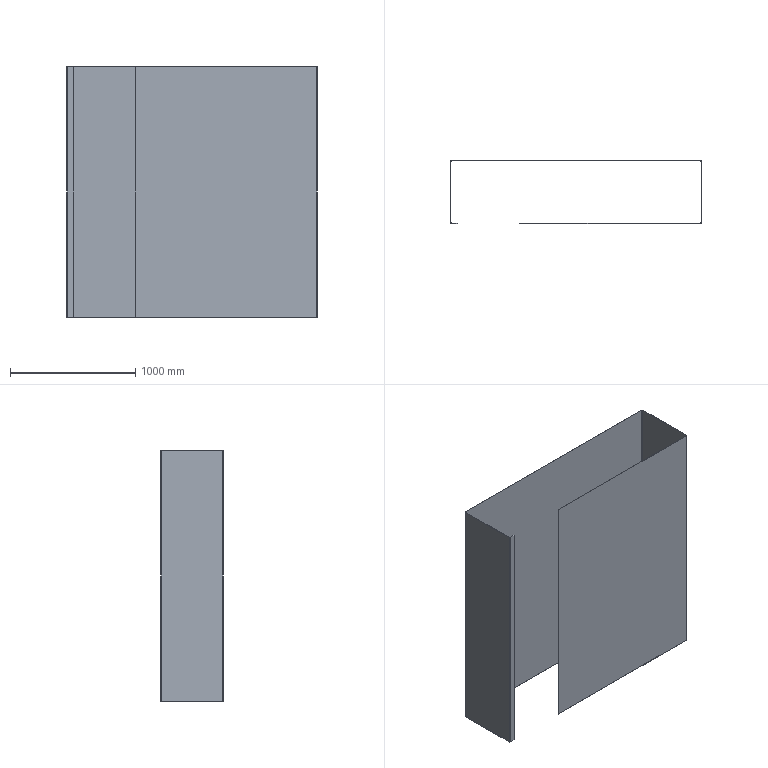Part | SolidWorks | features BaseBody 1 | 1 solid | 38 faces | box 2003 x 503 x 2000 mm | volume 13488385 mm3 | plane 30 | cylinder 8 | commonest cylinder face diameters 10 x4 13 x4
STEP:
#1=CARTESIAN_POINT('',(-995.,-500.,2000.));
#2=VERTEX_POINT('',#1);
#3=CARTESIAN_POINT('',(-995.,-501.5,2000.));
#4=VERTEX_POINT('',#3);
#5=CARTESIAN_POINT('',(-995.,-500.,2000.));
#6=DIRECTION('',(0.,-1.,0.));
#7=VECTOR('',#6,1000.);
#8=LINE('',#5,#7);
#9=EDGE_CURVE('',#2,#4,#8,.T.);
#10=ORIENTED_EDGE('',*,*,#9,.F.);
#11=CARTESIAN_POINT('',(-1000.,-495.,2000.));
#12=VERTEX_POINT('',#11);
#13=CARTESIAN_POINT('',(-995.,-495.,2000.));
#14=DIRECTION('',(0.,0.,1.));
#15=DIRECTION('',(1.,0.,0.));
#16=AXIS2_PLACEMENT_3D('',#13,#14,#15);
#17=CIRCLE('',#16,5.);
#18=EDGE_CURVE('',#12,#2,#17,.T.);
#19=ORIENTED_EDGE('',*,*,#18,.F.);
#20=CARTESIAN_POINT('',(-1001.5,-495.,2000.));
#21=VERTEX_POINT('',#20);
#22=CARTESIAN_POINT('',(-1001.5,-495.,2000.));
#23=DIRECTION('',(1.,0.,0.));
#24=VECTOR('',#23,1000.);
#25=LINE('',#22,#24);
#26=EDGE_CURVE('',#21,#12,#25,.T.);
#27=ORIENTED_EDGE('',*,*,#26,.F.);
#28=CARTESIAN_POINT('',(-995.,-495.,2000.));
#29=DIRECTION('',(0.,0.,1.));
#30=DIRECTION('',(1.,0.,0.));
#31=AXIS2_PLACEMENT_3D('',#28,#29,#30);
#32=CIRCLE('',#31,6.5);
#33=EDGE_CURVE('',#21,#4,#32,.T.);
#34=ORIENTED_EDGE('',*,*,#33,.T.);
#35=EDGE_LOOP('',(#10,#19,#27,#34));
#36=FACE_OUTER_BOUND('',#35,.T.);
#37=CARTESIAN_POINT('',(-995.,-500.,2000.));
#38=DIRECTION('',(0.,0.,1.));
#39=DIRECTION('',(1.,0.,0.));
#40=AXIS2_PLACEMENT_3D('',#37,#38,#39);
#41=PLANE('',#40);
#42=ADVANCED_FACE('',(#36),#41,.T.);
#43=CARTESIAN_POINT('',(-950.,-500.,2000.));
#44=VERTEX_POINT('',#43);
#45=CARTESIAN_POINT('',(-995.,-500.,2000.));
#46=DIRECTION('',(1.,0.,0.));
#47=VECTOR('',#46,1000.);
#48=LINE('',#45,#47);
#49=EDGE_CURVE('',#2,#44,#48,.T.);
#50=ORIENTED_EDGE('',*,*,#49,.F.);
#51=ORIENTED_EDGE('',*,*,#9,.T.);
#52=CARTESIAN_POINT('',(-950.,-501.5,2000.));
#53=VERTEX_POINT('',#52);
#54=CARTESIAN_POINT('',(-995.,-501.5,2000.));
#55=DIRECTION('',(1.,0.,0.));
#56=VECTOR('',#55,1000.);
#57=LINE('',#54,#56);
#58=EDGE_CURVE('',#4,#53,#57,.T.);
#59=ORIENTED_EDGE('',*,*,#58,.T.);
#60=CARTESIAN_POINT('',(-950.,-500.,2000.));
#61=DIRECTION('',(0.,-1.,0.));
#62=VECTOR('',#61,1000.);
#63=LINE('',#60,#62);
#64=EDGE_CURVE('',#44,#53,#63,.T.);
#65=ORIENTED_EDGE('',*,*,#64,.F.);
#66=EDGE_LOOP('',(#50,#51,#59,#65));
#67=FACE_OUTER_BOUND('',#66,.T.);
#68=CARTESIAN_POINT('',(-1001.5,-495.,2000.));
#69=DIRECTION('',(0.,0.,1.));
#70=DIRECTION('',(1.,0.,0.));
#71=AXIS2_PLACEMENT_3D('',#68,#69,#70);
#72=PLANE('',#71);
#73=ADVANCED_FACE('',(#67),#72,.T.);
#74=CARTESIAN_POINT('',(-1000.,-495.,0.));
#75=VERTEX_POINT('',#74);
#76=CARTESIAN_POINT('',(-1001.5,-495.,0.));
#77=VERTEX_POINT('',#76);
#78=CARTESIAN_POINT('',(-1000.,-495.,0.));
#79=DIRECTION('',(-1.,0.,0.));
#80=VECTOR('',#79,1000.);
#81=LINE('',#78,#80);
#82=EDGE_CURVE('',#75,#77,#81,.T.);
#83=ORIENTED_EDGE('',*,*,#82,.F.);
#84=CARTESIAN_POINT('',(-995.,-500.,0.));
#85=VERTEX_POINT('',#84);
#86=CARTESIAN_POINT('',(-995.,-495.,0.));
#87=DIRECTION('',(0.,0.,1.));
#88=DIRECTION('',(1.,0.,0.));
#89=AXIS2_PLACEMENT_3D('',#86,#87,#88);
#90=CIRCLE('',#89,5.);
#91=EDGE_CURVE('',#75,#85,#90,.T.);
#92=ORIENTED_EDGE('',*,*,#91,.T.);
#93=CARTESIAN_POINT('',(-995.,-501.5,0.));
#94=VERTEX_POINT('',#93);
#95=CARTESIAN_POINT('',(-995.,-501.5,0.));
#96=DIRECTION('',(0.,1.,0.));
#97=VECTOR('',#96,1000.);
#98=LINE('',#95,#97);
#99=EDGE_CURVE('',#94,#85,#98,.T.);
#100=ORIENTED_EDGE('',*,*,#99,.F.);
#101=CARTESIAN_POINT('',(-995.,-495.,0.));
#102=DIRECTION('',(0.,0.,1.));
#103=DIRECTION('',(1.,0.,0.));
#104=AXIS2_PLACEMENT_3D('',#101,#102,#103);
#105=CIRCLE('',#104,6.5);
#106=EDGE_CURVE('',#77,#94,#105,.T.);
#107=ORIENTED_EDGE('',*,*,#106,.F.);
#108=EDGE_LOOP('',(#83,#92,#100,#107));
#109=FACE_OUTER_BOUND('',#108,.T.);
#110=CARTESIAN_POINT('',(-1000.,-495.,0.));
#111=DIRECTION('',(0.,0.,-1.));
#112=DIRECTION('',(-1.,0.,0.));
#113=AXIS2_PLACEMENT_3D('',#110,#111,#112);
#114=PLANE('',#113);
#115=ADVANCED_FACE('',(#109),#114,.T.);
#116=CARTESIAN_POINT('',(-1000.,-5.,0.));
#117=VERTEX_POINT('',#116);
#118=CARTESIAN_POINT('',(-1000.,-5.,0.));
#119=DIRECTION('',(0.,-1.,0.));
#120=VECTOR('',#119,1000.);
#121=LINE('',#118,#120);
#122=EDGE_CURVE('',#117,#75,#121,.T.);
#123=ORIENTED_EDGE('',*,*,#122,.T.);
#124=ORIENTED_EDGE('',*,*,#82,.T.);
#125=CARTESIAN_POINT('',(-1001.5,-5.,0.));
#126=VERTEX_POINT('',#125);
#127=CARTESIAN_POINT('',(-1001.5,-5.,0.));
#128=DIRECTION('',(0.,-1.,0.));
#129=VECTOR('',#128,1000.);
#130=LINE('',#127,#129);
#131=EDGE_CURVE('',#126,#77,#130,.T.);
#132=ORIENTED_EDGE('',*,*,#131,.F.);
#133=CARTESIAN_POINT('',(-1001.5,-5.,0.));
#134=DIRECTION('',(1.,0.,0.));
#135=VECTOR('',#134,1000.);
#136=LINE('',#133,#135);
#137=EDGE_CURVE('',#126,#117,#136,.T.);
#138=ORIENTED_EDGE('',*,*,#137,.T.);
#139=EDGE_LOOP('',(#123,#124,#132,#138));
#140=FACE_OUTER_BOUND('',#139,.T.);
#141=CARTESIAN_POINT('',(-995.,-501.5,0.));
#142=DIRECTION('',(0.,0.,-1.));
#143=DIRECTION('',(-1.,0.,0.));
#144=AXIS2_PLACEMENT_3D('',#141,#142,#143);
#145=PLANE('',#144);
#146=ADVANCED_FACE('',(#140),#145,.T.);
#147=CARTESIAN_POINT('',(-1000.,-5.,2000.));
#148=VERTEX_POINT('',#147);
#149=CARTESIAN_POINT('',(-1001.5,-5.,2000.));
#150=VERTEX_POINT('',#149);
#151=CARTESIAN_POINT('',(-1000.,-5.,2000.));
#152=DIRECTION('',(-1.,0.,0.));
#153=VECTOR('',#152,1000.);
#154=LINE('',#151,#153);
#155=EDGE_CURVE('',#148,#150,#154,.T.);
#156=ORIENTED_EDGE('',*,*,#155,.F.);
#157=CARTESIAN_POINT('',(-995.,0.,2000.));
#158=VERTEX_POINT('',#157);
#159=CARTESIAN_POINT('',(-995.,-5.,2000.));
#160=DIRECTION('',(0.,0.,1.));
#161=DIRECTION('',(1.,0.,0.));
#162=AXIS2_PLACEMENT_3D('',#159,#160,#161);
#163=CIRCLE('',#162,5.);
#164=EDGE_CURVE('',#158,#148,#163,.T.);
#165=ORIENTED_EDGE('',*,*,#164,.F.);
#166=CARTESIAN_POINT('',(-995.,1.5,2000.));
#167=VERTEX_POINT('',#166);
#168=CARTESIAN_POINT('',(-995.,1.5,2000.));
#169=DIRECTION('',(0.,-1.,0.));
#170=VECTOR('',#169,1000.);
#171=LINE('',#168,#170);
#172=EDGE_CURVE('',#167,#158,#171,.T.);
#173=ORIENTED_EDGE('',*,*,#172,.F.);
#174=CARTESIAN_POINT('',(-995.,-5.,2000.));
#175=DIRECTION('',(0.,0.,1.));
#176=DIRECTION('',(1.,0.,0.));
#177=AXIS2_PLACEMENT_3D('',#174,#175,#176);
#178=CIRCLE('',#177,6.5);
#179=EDGE_CURVE('',#167,#150,#178,.T.);
#180=ORIENTED_EDGE('',*,*,#179,.T.);
#181=EDGE_LOOP('',(#156,#165,#173,#180));
#182=FACE_OUTER_BOUND('',#181,.T.);
#183=CARTESIAN_POINT('',(-1000.,-5.,2000.));
#184=DIRECTION('',(0.,0.,1.));
#185=DIRECTION('',(1.,0.,0.));
#186=AXIS2_PLACEMENT_3D('',#183,#184,#185);
#187=PLANE('',#186);
#188=ADVANCED_FACE('',(#182),#187,.T.);
#189=CARTESIAN_POINT('',(-1000.,-5.,2000.));
#190=DIRECTION('',(0.,-1.,0.));
#191=VECTOR('',#190,1000.);
#192=LINE('',#189,#191);
#193=EDGE_CURVE('',#148,#12,#192,.T.);
#194=ORIENTED_EDGE('',*,*,#193,.F.);
#195=ORIENTED_EDGE('',*,*,#155,.T.);
#196=CARTESIAN_POINT('',(-1001.5,-5.,2000.));
#197=DIRECTION('',(0.,-1.,0.));
#198=VECTOR('',#197,1000.);
#199=LINE('',#196,#198);
#200=EDGE_CURVE('',#150,#21,#199,.T.);
#201=ORIENTED_EDGE('',*,*,#200,.T.);
#202=ORIENTED_EDGE('',*,*,#26,.T.);
#203=EDGE_LOOP('',(#194,#195,#201,#202));
#204=FACE_OUTER_BOUND('',#203,.T.);
#205=CARTESIAN_POINT('',(-995.,1.5,2000.));
#206=DIRECTION('',(0.,0.,1.));
#207=DIRECTION('',(1.,0.,0.));
#208=AXIS2_PLACEMENT_3D('',#205,#206,#207);
#209=PLANE('',#208);
#210=ADVANCED_FACE('',(#204),#209,.T.);
#211=CARTESIAN_POINT('',(-995.,0.,0.));
#212=VERTEX_POINT('',#211);
#213=CARTESIAN_POINT('',(-995.,1.5,0.));
#214=VERTEX_POINT('',#213);
#215=CARTESIAN_POINT('',(-995.,0.,0.));
#216=DIRECTION('',(0.,1.,0.));
#217=VECTOR('',#216,1000.);
#218=LINE('',#215,#217);
#219=EDGE_CURVE('',#212,#214,#218,.T.);
#220=ORIENTED_EDGE('',*,*,#219,.F.);
#221=CARTESIAN_POINT('',(-995.,-5.,0.));
#222=DIRECTION('',(0.,0.,1.));
#223=DIRECTION('',(1.,0.,0.));
#224=AXIS2_PLACEMENT_3D('',#221,#222,#223);
#225=CIRCLE('',#224,5.);
#226=EDGE_CURVE('',#212,#117,#225,.T.);
#227=ORIENTED_EDGE('',*,*,#226,.T.);
#228=ORIENTED_EDGE('',*,*,#137,.F.);
#229=CARTESIAN_POINT('',(-995.,-5.,0.));
#230=DIRECTION('',(0.,0.,1.));
#231=DIRECTION('',(1.,0.,0.));
#232=AXIS2_PLACEMENT_3D('',#229,#230,#231);
#233=CIRCLE('',#232,6.5);
#234=EDGE_CURVE('',#214,#126,#233,.T.);
#235=ORIENTED_EDGE('',*,*,#234,.F.);
#236=EDGE_LOOP('',(#220,#227,#228,#235));
#237=FACE_OUTER_BOUND('',#236,.T.);
#238=CARTESIAN_POINT('',(-995.,0.,0.));
#239=DIRECTION('',(0.,0.,-1.));
#240=DIRECTION('',(-1.,0.,0.));
#241=AXIS2_PLACEMENT_3D('',#238,#239,#240);
#242=PLANE('',#241);
#243=ADVANCED_FACE('',(#237),#242,.T.);
#244=CARTESIAN_POINT('',(995.,0.,0.));
#245=VERTEX_POINT('',#244);
#246=CARTESIAN_POINT('',(-995.,0.,0.));
#247=DIRECTION('',(-1.,0.,0.));
#248=VECTOR('',#247,1000.);
#249=LINE('',#246,#248);
#250=EDGE_CURVE('',#245,#212,#249,.T.);
#251=ORIENTED_EDGE('',*,*,#250,.T.);
#252=ORIENTED_EDGE('',*,*,#219,.T.);
#253=CARTESIAN_POINT('',(995.,1.5,0.));
#254=VERTEX_POINT('',#253);
#255=CARTESIAN_POINT('',(-995.,1.5,0.));
#256=DIRECTION('',(-1.,0.,0.));
#257=VECTOR('',#256,1000.);
#258=LINE('',#255,#257);
#259=EDGE_CURVE('',#254,#214,#258,.T.);
#260=ORIENTED_EDGE('',*,*,#259,.F.);
#261=CARTESIAN_POINT('',(995.,1.5,0.));
#262=DIRECTION('',(0.,-1.,0.));
#263=VECTOR('',#262,1000.);
#264=LINE('',#261,#263);
#265=EDGE_CURVE('',#254,#245,#264,.T.);
#266=ORIENTED_EDGE('',*,*,#265,.T.);
#267=EDGE_LOOP('',(#251,#252,#260,#266));
#268=FACE_OUTER_BOUND('',#267,.T.);
#269=CARTESIAN_POINT('',(-1001.5,-5.,0.));
#270=DIRECTION('',(0.,0.,-1.));
#271=DIRECTION('',(-1.,0.,0.));
#272=AXIS2_PLACEMENT_3D('',#269,#270,#271);
#273=PLANE('',#272);
#274=ADVANCED_FACE('',(#268),#273,.T.);
#275=CARTESIAN_POINT('',(995.,0.,2000.));
#276=VERTEX_POINT('',#275);
#277=CARTESIAN_POINT('',(995.,1.5,2000.));
#278=VERTEX_POINT('',#277);
#279=CARTESIAN_POINT('',(995.,0.,2000.));
#280=DIRECTION('',(0.,1.,0.));
#281=VECTOR('',#280,1000.);
#282=LINE('',#279,#281);
#283=EDGE_CURVE('',#276,#278,#282,.T.);
#284=ORIENTED_EDGE('',*,*,#283,.F.);
#285=CARTESIAN_POINT('',(1000.,-5.,2000.));
#286=VERTEX_POINT('',#285);
#287=CARTESIAN_POINT('',(995.,-5.,2000.));
#288=DIRECTION('',(0.,0.,1.));
#289=DIRECTION('',(-1.,0.,0.));
#290=AXIS2_PLACEMENT_3D('',#287,#288,#289);
#291=CIRCLE('',#290,5.);
#292=EDGE_CURVE('',#286,#276,#291,.T.);
#293=ORIENTED_EDGE('',*,*,#292,.F.);
#294=CARTESIAN_POINT('',(1001.5,-5.,2000.));
#295=VERTEX_POINT('',#294);
#296=CARTESIAN_POINT('',(1001.5,-5.,2000.));
#297=DIRECTION('',(-1.,0.,0.));
#298=VECTOR('',#297,1000.);
#299=LINE('',#296,#298);
#300=EDGE_CURVE('',#295,#286,#299,.T.);
#301=ORIENTED_EDGE('',*,*,#300,.F.);
#302=CARTESIAN_POINT('',(995.,-5.,2000.));
#303=DIRECTION('',(0.,0.,1.));
#304=DIRECTION('',(1.,0.,0.));
#305=AXIS2_PLACEMENT_3D('',#302,#303,#304);
#306=CIRCLE('',#305,6.5);
#307=EDGE_CURVE('',#295,#278,#306,.T.);
#308=ORIENTED_EDGE('',*,*,#307,.T.);
#309=EDGE_LOOP('',(#284,#293,#301,#308));
#310=FACE_OUTER_BOUND('',#309,.T.);
#311=CARTESIAN_POINT('',(995.,0.,2000.));
#312=DIRECTION('',(0.,0.,1.));
#313=DIRECTION('',(1.,0.,0.));
#314=AXIS2_PLACEMENT_3D('',#311,#312,#313);
#315=PLANE('',#314);
#316=ADVANCED_FACE('',(#310),#315,.T.);
#317=CARTESIAN_POINT('',(-995.,0.,2000.));
#318=DIRECTION('',(-1.,0.,0.));
#319=VECTOR('',#318,1000.);
#320=LINE('',#317,#319);
#321=EDGE_CURVE('',#276,#158,#320,.T.);
#322=ORIENTED_EDGE('',*,*,#321,.F.);
#323=ORIENTED_EDGE('',*,*,#283,.T.);
#324=CARTESIAN_POINT('',(-995.,1.5,2000.));
#325=DIRECTION('',(-1.,0.,0.));
#326=VECTOR('',#325,1000.);
#327=LINE('',#324,#326);
#328=EDGE_CURVE('',#278,#167,#327,.T.);
#329=ORIENTED_EDGE('',*,*,#328,.T.);
#330=ORIENTED_EDGE('',*,*,#172,.T.);
#331=EDGE_LOOP('',(#322,#323,#329,#330));
#332=FACE_OUTER_BOUND('',#331,.T.);
#333=CARTESIAN_POINT('',(1001.5,-5.,2000.));
#334=DIRECTION('',(0.,0.,1.));
#335=DIRECTION('',(1.,0.,0.));
#336=AXIS2_PLACEMENT_3D('',#333,#334,#335);
#337=PLANE('',#336);
#338=ADVANCED_FACE('',(#332),#337,.T.);
#339=CARTESIAN_POINT('',(1000.,-5.,0.));
#340=VERTEX_POINT('',#339);
#341=CARTESIAN_POINT('',(1001.5,-5.,0.));
#342=VERTEX_POINT('',#341);
#343=CARTESIAN_POINT('',(1000.,-5.,0.));
#344=DIRECTION('',(1.,0.,0.));
#345=VECTOR('',#344,1000.);
#346=LINE('',#343,#345);
#347=EDGE_CURVE('',#340,#342,#346,.T.);
#348=ORIENTED_EDGE('',*,*,#347,.F.);
#349=CARTESIAN_POINT('',(995.,-5.,0.));
#350=DIRECTION('',(0.,0.,1.));
#351=DIRECTION('',(-1.,0.,0.));
#352=AXIS2_PLACEMENT_3D('',#349,#350,#351);
#353=CIRCLE('',#352,5.);
#354=EDGE_CURVE('',#340,#245,#353,.T.);
#355=ORIENTED_EDGE('',*,*,#354,.T.);
#356=ORIENTED_EDGE('',*,*,#265,.F.);
#357=CARTESIAN_POINT('',(995.,-5.,0.));
#358=DIRECTION('',(0.,0.,1.));
#359=DIRECTION('',(1.,0.,0.));
#360=AXIS2_PLACEMENT_3D('',#357,#358,#359);
#361=CIRCLE('',#360,6.5);
#362=EDGE_CURVE('',#342,#254,#361,.T.);
#363=ORIENTED_EDGE('',*,*,#362,.F.);
#364=EDGE_LOOP('',(#348,#355,#356,#363));
#365=FACE_OUTER_BOUND('',#364,.T.);
#366=CARTESIAN_POINT('',(1000.,-5.,0.));
#367=DIRECTION('',(0.,0.,-1.));
#368=DIRECTION('',(-1.,0.,0.));
#369=AXIS2_PLACEMENT_3D('',#366,#367,#368);
#370=PLANE('',#369);
#371=ADVANCED_FACE('',(#365),#370,.T.);
#372=CARTESIAN_POINT('',(1000.,-495.,0.));
#373=VERTEX_POINT('',#372);
#374=CARTESIAN_POINT('',(1000.,-5.,0.));
#375=DIRECTION('',(0.,1.,0.));
#376=VECTOR('',#375,1000.);
#377=LINE('',#374,#376);
#378=EDGE_CURVE('',#373,#340,#377,.T.);
#379=ORIENTED_EDGE('',*,*,#378,.T.);
#380=ORIENTED_EDGE('',*,*,#347,.T.);
#381=CARTESIAN_POINT('',(1001.5,-495.,0.));
#382=VERTEX_POINT('',#381);
#383=CARTESIAN_POINT('',(1001.5,-5.,0.));
#384=DIRECTION('',(0.,1.,0.));
#385=VECTOR('',#384,1000.);
#386=LINE('',#383,#385);
#387=EDGE_CURVE('',#382,#342,#386,.T.);
#388=ORIENTED_EDGE('',*,*,#387,.F.);
#389=CARTESIAN_POINT('',(1001.5,-495.,0.));
#390=DIRECTION('',(-1.,0.,0.));
#391=VECTOR('',#390,1000.);
#392=LINE('',#389,#391);
#393=EDGE_CURVE('',#382,#373,#392,.T.);
#394=ORIENTED_EDGE('',*,*,#393,.T.);
#395=EDGE_LOOP('',(#379,#380,#388,#394));
#396=FACE_OUTER_BOUND('',#395,.T.);
#397=CARTESIAN_POINT('',(995.,1.5,0.));
#398=DIRECTION('',(0.,0.,-1.));
#399=DIRECTION('',(-1.,0.,0.));
#400=AXIS2_PLACEMENT_3D('',#397,#398,#399);
#401=PLANE('',#400);
#402=ADVANCED_FACE('',(#396),#401,.T.);
#403=CARTESIAN_POINT('',(1000.,-495.,2000.));
#404=VERTEX_POINT('',#403);
#405=CARTESIAN_POINT('',(1001.5,-495.,2000.));
#406=VERTEX_POINT('',#405);
#407=CARTESIAN_POINT('',(1000.,-495.,2000.));
#408=DIRECTION('',(1.,0.,0.));
#409=VECTOR('',#408,1000.);
#410=LINE('',#407,#409);
#411=EDGE_CURVE('',#404,#406,#410,.T.);
#412=ORIENTED_EDGE('',*,*,#411,.F.);
#413=CARTESIAN_POINT('',(995.,-500.,2000.));
#414=VERTEX_POINT('',#413);
#415=CARTESIAN_POINT('',(995.,-495.,2000.));
#416=DIRECTION('',(0.,0.,1.));
#417=DIRECTION('',(1.,0.,0.));
#418=AXIS2_PLACEMENT_3D('',#415,#416,#417);
#419=CIRCLE('',#418,5.);
#420=EDGE_CURVE('',#414,#404,#419,.T.);
#421=ORIENTED_EDGE('',*,*,#420,.F.);
#422=CARTESIAN_POINT('',(995.,-501.5,2000.));
#423=VERTEX_POINT('',#422);
#424=CARTESIAN_POINT('',(995.,-501.5,2000.));
#425=DIRECTION('',(0.,1.,0.));
#426=VECTOR('',#425,1000.);
#427=LINE('',#424,#426);
#428=EDGE_CURVE('',#423,#414,#427,.T.);
#429=ORIENTED_EDGE('',*,*,#428,.F.);
#430=CARTESIAN_POINT('',(995.,-495.,2000.));
#431=DIRECTION('',(0.,0.,1.));
#432=DIRECTION('',(1.,0.,0.));
#433=AXIS2_PLACEMENT_3D('',#430,#431,#432);
#434=CIRCLE('',#433,6.5);
#435=EDGE_CURVE('',#423,#406,#434,.T.);
#436=ORIENTED_EDGE('',*,*,#435,.T.);
#437=EDGE_LOOP('',(#412,#421,#429,#436));
#438=FACE_OUTER_BOUND('',#437,.T.);
#439=CARTESIAN_POINT('',(1000.,-495.,2000.));
#440=DIRECTION('',(0.,0.,1.));
#441=DIRECTION('',(1.,0.,0.));
#442=AXIS2_PLACEMENT_3D('',#439,#440,#441);
#443=PLANE('',#442);
#444=ADVANCED_FACE('',(#438),#443,.T.);
#445=CARTESIAN_POINT('',(1000.,-5.,2000.));
#446=DIRECTION('',(0.,1.,0.));
#447=VECTOR('',#446,1000.);
#448=LINE('',#445,#447);
#449=EDGE_CURVE('',#404,#286,#448,.T.);
#450=ORIENTED_EDGE('',*,*,#449,.F.);
#451=ORIENTED_EDGE('',*,*,#411,.T.);
#452=CARTESIAN_POINT('',(1001.5,-5.,2000.));
#453=DIRECTION('',(0.,1.,0.));
#454=VECTOR('',#453,1000.);
#455=LINE('',#452,#454);
#456=EDGE_CURVE('',#406,#295,#455,.T.);
#457=ORIENTED_EDGE('',*,*,#456,.T.);
#458=ORIENTED_EDGE('',*,*,#300,.T.);
#459=EDGE_LOOP('',(#450,#451,#457,#458));
#460=FACE_OUTER_BOUND('',#459,.T.);
#461=CARTESIAN_POINT('',(995.,-501.5,2000.));
#462=DIRECTION('',(0.,0.,1.));
#463=DIRECTION('',(1.,0.,0.));
#464=AXIS2_PLACEMENT_3D('',#461,#462,#463);
#465=PLANE('',#464);
#466=ADVANCED_FACE('',(#460),#465,.T.);
#467=CARTESIAN_POINT('',(995.,-500.,0.));
#468=VERTEX_POINT('',#467);
#469=CARTESIAN_POINT('',(995.,-501.5,0.));
#470=VERTEX_POINT('',#469);
#471=CARTESIAN_POINT('',(995.,-500.,0.));
#472=DIRECTION('',(0.,-1.,0.));
#473=VECTOR('',#472,1000.);
#474=LINE('',#471,#473);
#475=EDGE_CURVE('',#468,#470,#474,.T.);
#476=ORIENTED_EDGE('',*,*,#475,.F.);
#477=CARTESIAN_POINT('',(995.,-495.,0.));
#478=DIRECTION('',(0.,0.,1.));
#479=DIRECTION('',(1.,0.,0.));
#480=AXIS2_PLACEMENT_3D('',#477,#478,#479);
#481=CIRCLE('',#480,5.);
#482=EDGE_CURVE('',#468,#373,#481,.T.);
#483=ORIENTED_EDGE('',*,*,#482,.T.);
#484=ORIENTED_EDGE('',*,*,#393,.F.);
#485=CARTESIAN_POINT('',(995.,-495.,0.));
#486=DIRECTION('',(0.,0.,1.));
#487=DIRECTION('',(1.,0.,0.));
#488=AXIS2_PLACEMENT_3D('',#485,#486,#487);
#489=CIRCLE('',#488,6.5);
#490=EDGE_CURVE('',#470,#382,#489,.T.);
#491=ORIENTED_EDGE('',*,*,#490,.F.);
#492=EDGE_LOOP('',(#476,#483,#484,#491));
#493=FACE_OUTER_BOUND('',#492,.T.);
#494=CARTESIAN_POINT('',(995.,-500.,0.));
#495=DIRECTION('',(0.,0.,-1.));
#496=DIRECTION('',(-1.,0.,0.));
#497=AXIS2_PLACEMENT_3D('',#494,#495,#496);
#498=PLANE('',#497);
#499=ADVANCED_FACE('',(#493),#498,.T.);
#500=CARTESIAN_POINT('',(-450.,-500.,0.));
#501=VERTEX_POINT('',#500);
#502=CARTESIAN_POINT('',(-450.,-500.,0.));
#503=DIRECTION('',(1.,0.,0.));
#504=VECTOR('',#503,1000.);
#505=LINE('',#502,#504);
#506=EDGE_CURVE('',#501,#468,#505,.T.);
#507=ORIENTED_EDGE('',*,*,#506,.T.);
#508=ORIENTED_EDGE('',*,*,#475,.T.);
#509=CARTESIAN_POINT('',(-450.,-501.5,0.));
#510=VERTEX_POINT('',#509);
#511=CARTESIAN_POINT('',(-450.,-501.5,0.));
#512=DIRECTION('',(1.,0.,0.));
#513=VECTOR('',#512,1000.);
#514=LINE('',#511,#513);
#515=EDGE_CURVE('',#510,#470,#514,.T.);
#516=ORIENTED_EDGE('',*,*,#515,.F.);
#517=CARTESIAN_POINT('',(-450.,-501.5,0.));
#518=DIRECTION('',(0.,1.,0.));
#519=VECTOR('',#518,1000.);
#520=LINE('',#517,#519);
#521=EDGE_CURVE('',#510,#501,#520,.T.);
#522=ORIENTED_EDGE('',*,*,#521,.T.);
#523=EDGE_LOOP('',(#507,#508,#516,#522));
#524=FACE_OUTER_BOUND('',#523,.T.);
#525=CARTESIAN_POINT('',(1001.5,-495.,0.));
#526=DIRECTION('',(0.,0.,-1.));
#527=DIRECTION('',(-1.,0.,0.));
#528=AXIS2_PLACEMENT_3D('',#525,#526,#527);
#529=PLANE('',#528);
#530=ADVANCED_FACE('',(#524),#529,.T.);
#531=CARTESIAN_POINT('',(-950.,-501.5,0.));
#532=VERTEX_POINT('',#531);
#533=CARTESIAN_POINT('',(-995.,-501.5,0.));
#534=DIRECTION('',(1.,0.,0.));
#535=VECTOR('',#534,1000.);
#536=LINE('',#533,#535);
#537=EDGE_CURVE('',#94,#532,#536,.T.);
#538=ORIENTED_EDGE('',*,*,#537,.T.);
#539=CARTESIAN_POINT('',(-950.,-501.5,2000.));
#540=DIRECTION('',(0.,0.,-1.));
#541=VECTOR('',#540,1000.);
#542=LINE('',#539,#541);
#543=EDGE_CURVE('',#53,#532,#542,.T.);
#544=ORIENTED_EDGE('',*,*,#543,.F.);
#545=ORIENTED_EDGE('',*,*,#58,.F.);
#546=CARTESIAN_POINT('',(-995.,-501.5,2000.));
#547=DIRECTION('',(0.,0.,-1.));
#548=VECTOR('',#547,1000.);
#549=LINE('',#546,#548);
#550=EDGE_CURVE('',#4,#94,#549,.T.);
#551=ORIENTED_EDGE('',*,*,#550,.T.);
#552=EDGE_LOOP('',(#538,#544,#545,#551));
#553=FACE_OUTER_BOUND('',#552,.T.);
#554=CARTESIAN_POINT('',(-995.,-501.5,2000.));
#555=DIRECTION('',(0.,1.,0.));
#556=DIRECTION('',(0.,0.,1.));
#557=AXIS2_PLACEMENT_3D('',#554,#555,#556);
#558=PLANE('',#557);
#559=ADVANCED_FACE('',(#553),#558,.F.);
#560=CARTESIAN_POINT('',(-950.,-500.,0.));
#561=VERTEX_POINT('',#560);
#562=CARTESIAN_POINT('',(-950.,-500.,0.));
#563=DIRECTION('',(0.,-1.,0.));
#564=VECTOR('',#563,1000.);
#565=LINE('',#562,#564);
#566=EDGE_CURVE('',#561,#532,#565,.T.);
#567=ORIENTED_EDGE('',*,*,#566,.F.);
#568=CARTESIAN_POINT('',(-950.,-500.,2000.));
#569=DIRECTION('',(0.,0.,-1.));
#570=VECTOR('',#569,1000.);
#571=LINE('',#568,#570);
#572=EDGE_CURVE('',#44,#561,#571,.T.);
#573=ORIENTED_EDGE('',*,*,#572,.F.);
#574=ORIENTED_EDGE('',*,*,#64,.T.);
#575=ORIENTED_EDGE('',*,*,#543,.T.);
#576=EDGE_LOOP('',(#567,#573,#574,#575));
#577=FACE_OUTER_BOUND('',#576,.T.);
#578=CARTESIAN_POINT('',(-950.,-500.,2000.));
#579=DIRECTION('',(1.,0.,0.));
#580=DIRECTION('',(0.,0.,-1.));
#581=AXIS2_PLACEMENT_3D('',#578,#579,#580);
#582=PLANE('',#581);
#583=ADVANCED_FACE('',(#577),#582,.T.);
#584=CARTESIAN_POINT('',(-995.,-500.,0.));
#585=DIRECTION('',(1.,0.,0.));
#586=VECTOR('',#585,1000.);
#587=LINE('',#584,#586);
#588=EDGE_CURVE('',#85,#561,#587,.T.);
#589=ORIENTED_EDGE('',*,*,#588,.F.);
#590=CARTESIAN_POINT('',(-995.,-500.,2000.));
#591=DIRECTION('',(0.,0.,-1.));
#592=VECTOR('',#591,1000.);
#593=LINE('',#590,#592);
#594=EDGE_CURVE('',#2,#85,#593,.T.);
#595=ORIENTED_EDGE('',*,*,#594,.F.);
#596=ORIENTED_EDGE('',*,*,#49,.T.);
#597=ORIENTED_EDGE('',*,*,#572,.T.);
#598=EDGE_LOOP('',(#589,#595,#596,#597));
#599=FACE_OUTER_BOUND('',#598,.T.);
#600=CARTESIAN_POINT('',(-995.,-500.,2000.));
#601=DIRECTION('',(0.,1.,0.));
#602=DIRECTION('',(0.,0.,1.));
#603=AXIS2_PLACEMENT_3D('',#600,#601,#602);
#604=PLANE('',#603);
#605=ADVANCED_FACE('',(#599),#604,.T.);
#606=ORIENTED_EDGE('',*,*,#91,.F.);
#607=CARTESIAN_POINT('',(-1000.,-495.,2000.));
#608=DIRECTION('',(0.,0.,-1.));
#609=VECTOR('',#608,1000.);
#610=LINE('',#607,#609);
#611=EDGE_CURVE('',#12,#75,#610,.T.);
#612=ORIENTED_EDGE('',*,*,#611,.F.);
#613=ORIENTED_EDGE('',*,*,#18,.T.);
#614=ORIENTED_EDGE('',*,*,#594,.T.);
#615=EDGE_LOOP('',(#606,#612,#613,#614));
#616=FACE_OUTER_BOUND('',#615,.T.);
#617=CARTESIAN_POINT('',(-995.,-495.,2000.));
#618=DIRECTION('',(0.,0.,-1.));
#619=DIRECTION('',(-1.,0.,0.));
#620=AXIS2_PLACEMENT_3D('',#617,#618,#619);
#621=CYLINDRICAL_SURFACE('',#620,5.);
#622=ADVANCED_FACE('',(#616),#621,.F.);
#623=ORIENTED_EDGE('',*,*,#122,.F.);
#624=CARTESIAN_POINT('',(-1000.,-5.,2000.));
#625=DIRECTION('',(0.,0.,-1.));
#626=VECTOR('',#625,1000.);
#627=LINE('',#624,#626);
#628=EDGE_CURVE('',#148,#117,#627,.T.);
#629=ORIENTED_EDGE('',*,*,#628,.F.);
#630=ORIENTED_EDGE('',*,*,#193,.T.);
#631=ORIENTED_EDGE('',*,*,#611,.T.);
#632=EDGE_LOOP('',(#623,#629,#630,#631));
#633=FACE_OUTER_BOUND('',#632,.T.);
#634=CARTESIAN_POINT('',(-1000.,-5.,2000.));
#635=DIRECTION('',(1.,0.,0.));
#636=DIRECTION('',(0.,1.,0.));
#637=AXIS2_PLACEMENT_3D('',#634,#635,#636);
#638=PLANE('',#637);
#639=ADVANCED_FACE('',(#633),#638,.T.);
#640=ORIENTED_EDGE('',*,*,#226,.F.);
#641=CARTESIAN_POINT('',(-995.,0.,2000.));
#642=DIRECTION('',(0.,0.,-1.));
#643=VECTOR('',#642,1000.);
#644=LINE('',#641,#643);
#645=EDGE_CURVE('',#158,#212,#644,.T.);
#646=ORIENTED_EDGE('',*,*,#645,.F.);
#647=ORIENTED_EDGE('',*,*,#164,.T.);
#648=ORIENTED_EDGE('',*,*,#628,.T.);
#649=EDGE_LOOP('',(#640,#646,#647,#648));
#650=FACE_OUTER_BOUND('',#649,.T.);
#651=CARTESIAN_POINT('',(-995.,-5.,2000.));
#652=DIRECTION('',(0.,0.,-1.));
#653=DIRECTION('',(-1.,0.,0.));
#654=AXIS2_PLACEMENT_3D('',#651,#652,#653);
#655=CYLINDRICAL_SURFACE('',#654,5.);
#656=ADVANCED_FACE('',(#650),#655,.F.);
#657=ORIENTED_EDGE('',*,*,#250,.F.);
#658=CARTESIAN_POINT('',(995.,0.,2000.));
#659=DIRECTION('',(0.,0.,-1.));
#660=VECTOR('',#659,1000.);
#661=LINE('',#658,#660);
#662=EDGE_CURVE('',#276,#245,#661,.T.);
#663=ORIENTED_EDGE('',*,*,#662,.F.);
#664=ORIENTED_EDGE('',*,*,#321,.T.);
#665=ORIENTED_EDGE('',*,*,#645,.T.);
#666=EDGE_LOOP('',(#657,#663,#664,#665));
#667=FACE_OUTER_BOUND('',#666,.T.);
#668=CARTESIAN_POINT('',(-995.,0.,2000.));
#669=DIRECTION('',(0.,-1.,0.));
#670=DIRECTION('',(1.,0.,0.));
#671=AXIS2_PLACEMENT_3D('',#668,#669,#670);
#672=PLANE('',#671);
#673=ADVANCED_FACE('',(#667),#672,.T.);
#674=ORIENTED_EDGE('',*,*,#354,.F.);
#675=CARTESIAN_POINT('',(1000.,-5.,2000.));
#676=DIRECTION('',(0.,0.,-1.));
#677=VECTOR('',#676,1000.);
#678=LINE('',#675,#677);
#679=EDGE_CURVE('',#286,#340,#678,.T.);
#680=ORIENTED_EDGE('',*,*,#679,.F.);
#681=ORIENTED_EDGE('',*,*,#292,.T.);
#682=ORIENTED_EDGE('',*,*,#662,.T.);
#683=EDGE_LOOP('',(#674,#680,#681,#682));
#684=FACE_OUTER_BOUND('',#683,.T.);
#685=CARTESIAN_POINT('',(995.,-5.,2000.));
#686=DIRECTION('',(0.,0.,-1.));
#687=DIRECTION('',(-1.,0.,0.));
#688=AXIS2_PLACEMENT_3D('',#685,#686,#687);
#689=CYLINDRICAL_SURFACE('',#688,5.);
#690=ADVANCED_FACE('',(#684),#689,.F.);
#691=ORIENTED_EDGE('',*,*,#378,.F.);
#692=CARTESIAN_POINT('',(1000.,-495.,2000.));
#693=DIRECTION('',(0.,0.,-1.));
#694=VECTOR('',#693,1000.);
#695=LINE('',#692,#694);
#696=EDGE_CURVE('',#404,#373,#695,.T.);
#697=ORIENTED_EDGE('',*,*,#696,.F.);
#698=ORIENTED_EDGE('',*,*,#449,.T.);
#699=ORIENTED_EDGE('',*,*,#679,.T.);
#700=EDGE_LOOP('',(#691,#697,#698,#699));
#701=FACE_OUTER_BOUND('',#700,.T.);
#702=CARTESIAN_POINT('',(1000.,-5.,2000.));
#703=DIRECTION('',(-1.,0.,0.));
#704=DIRECTION('',(0.,0.,1.));
#705=AXIS2_PLACEMENT_3D('',#702,#703,#704);
#706=PLANE('',#705);
#707=ADVANCED_FACE('',(#701),#706,.T.);
#708=ORIENTED_EDGE('',*,*,#482,.F.);
#709=CARTESIAN_POINT('',(995.,-500.,2000.));
#710=DIRECTION('',(0.,0.,-1.));
#711=VECTOR('',#710,1000.);
#712=LINE('',#709,#711);
#713=EDGE_CURVE('',#414,#468,#712,.T.);
#714=ORIENTED_EDGE('',*,*,#713,.F.);
#715=ORIENTED_EDGE('',*,*,#420,.T.);
#716=ORIENTED_EDGE('',*,*,#696,.T.);
#717=EDGE_LOOP('',(#708,#714,#715,#716));
#718=FACE_OUTER_BOUND('',#717,.T.);
#719=CARTESIAN_POINT('',(995.,-495.,2000.));
#720=DIRECTION('',(0.,0.,-1.));
#721=DIRECTION('',(-1.,0.,0.));
#722=AXIS2_PLACEMENT_3D('',#719,#720,#721);
#723=CYLINDRICAL_SURFACE('',#722,5.);
#724=ADVANCED_FACE('',(#718),#723,.F.);
#725=ORIENTED_EDGE('',*,*,#506,.F.);
#726=CARTESIAN_POINT('',(-450.,-500.,2000.));
#727=VERTEX_POINT('',#726);
#728=CARTESIAN_POINT('',(-450.,-500.,2000.));
#729=DIRECTION('',(0.,0.,-1.));
#730=VECTOR('',#729,1000.);
#731=LINE('',#728,#730);
#732=EDGE_CURVE('',#727,#501,#731,.T.);
#733=ORIENTED_EDGE('',*,*,#732,.F.);
#734=CARTESIAN_POINT('',(-450.,-500.,2000.));
#735=DIRECTION('',(1.,0.,0.));
#736=VECTOR('',#735,1000.);
#737=LINE('',#734,#736);
#738=EDGE_CURVE('',#727,#414,#737,.T.);
#739=ORIENTED_EDGE('',*,*,#738,.T.);
#740=ORIENTED_EDGE('',*,*,#713,.T.);
#741=EDGE_LOOP('',(#725,#733,#739,#740));
#742=FACE_OUTER_BOUND('',#741,.T.);
#743=CARTESIAN_POINT('',(-450.,-500.,2000.));
#744=DIRECTION('',(0.,1.,0.));
#745=DIRECTION('',(-1.,0.,0.));
#746=AXIS2_PLACEMENT_3D('',#743,#744,#745);
#747=PLANE('',#746);
#748=ADVANCED_FACE('',(#742),#747,.T.);
#749=ORIENTED_EDGE('',*,*,#521,.F.);
#750=CARTESIAN_POINT('',(-450.,-501.5,2000.));
#751=VERTEX_POINT('',#750);
#752=CARTESIAN_POINT('',(-450.,-501.5,2000.));
#753=DIRECTION('',(0.,0.,-1.));
#754=VECTOR('',#753,1000.);
#755=LINE('',#752,#754);
#756=EDGE_CURVE('',#751,#510,#755,.T.);
#757=ORIENTED_EDGE('',*,*,#756,.F.);
#758=CARTESIAN_POINT('',(-450.,-501.5,2000.));
#759=DIRECTION('',(0.,1.,0.));
#760=VECTOR('',#759,1000.);
#761=LINE('',#758,#760);
#762=EDGE_CURVE('',#751,#727,#761,.T.);
#763=ORIENTED_EDGE('',*,*,#762,.T.);
#764=ORIENTED_EDGE('',*,*,#732,.T.);
#765=EDGE_LOOP('',(#749,#757,#763,#764));
#766=FACE_OUTER_BOUND('',#765,.T.);
#767=CARTESIAN_POINT('',(-450.,-501.5,2000.));
#768=DIRECTION('',(-1.,0.,0.));
#769=DIRECTION('',(0.,0.,1.));
#770=AXIS2_PLACEMENT_3D('',#767,#768,#769);
#771=PLANE('',#770);
#772=ADVANCED_FACE('',(#766),#771,.T.);
#773=ORIENTED_EDGE('',*,*,#515,.T.);
#774=CARTESIAN_POINT('',(995.,-501.5,2000.));
#775=DIRECTION('',(0.,0.,-1.));
#776=VECTOR('',#775,1000.);
#777=LINE('',#774,#776);
#778=EDGE_CURVE('',#423,#470,#777,.T.);
#779=ORIENTED_EDGE('',*,*,#778,.F.);
#780=CARTESIAN_POINT('',(-450.,-501.5,2000.));
#781=DIRECTION('',(1.,0.,0.));
#782=VECTOR('',#781,1000.);
#783=LINE('',#780,#782);
#784=EDGE_CURVE('',#751,#423,#783,.T.);
#785=ORIENTED_EDGE('',*,*,#784,.F.);
#786=ORIENTED_EDGE('',*,*,#756,.T.);
#787=EDGE_LOOP('',(#773,#779,#785,#786));
#788=FACE_OUTER_BOUND('',#787,.T.);
#789=CARTESIAN_POINT('',(-450.,-501.5,2000.));
#790=DIRECTION('',(0.,1.,0.));
#791=DIRECTION('',(-1.,0.,0.));
#792=AXIS2_PLACEMENT_3D('',#789,#790,#791);
#793=PLANE('',#792);
#794=ADVANCED_FACE('',(#788),#793,.F.);
#795=ORIENTED_EDGE('',*,*,#490,.T.);
#796=CARTESIAN_POINT('',(1001.5,-495.,2000.));
#797=DIRECTION('',(0.,0.,-1.));
#798=VECTOR('',#797,1000.);
#799=LINE('',#796,#798);
#800=EDGE_CURVE('',#406,#382,#799,.T.);
#801=ORIENTED_EDGE('',*,*,#800,.F.);
#802=ORIENTED_EDGE('',*,*,#435,.F.);
#803=ORIENTED_EDGE('',*,*,#778,.T.);
#804=EDGE_LOOP('',(#795,#801,#802,#803));
#805=FACE_OUTER_BOUND('',#804,.T.);
#806=CARTESIAN_POINT('',(995.,-495.,2000.));
#807=DIRECTION('',(0.,0.,-1.));
#808=DIRECTION('',(-1.,0.,0.));
#809=AXIS2_PLACEMENT_3D('',#806,#807,#808);
#810=CYLINDRICAL_SURFACE('',#809,6.5);
#811=ADVANCED_FACE('',(#805),#810,.T.);
#812=ORIENTED_EDGE('',*,*,#387,.T.);
#813=CARTESIAN_POINT('',(1001.5,-5.,2000.));
#814=DIRECTION('',(0.,0.,-1.));
#815=VECTOR('',#814,1000.);
#816=LINE('',#813,#815);
#817=EDGE_CURVE('',#295,#342,#816,.T.);
#818=ORIENTED_EDGE('',*,*,#817,.F.);
#819=ORIENTED_EDGE('',*,*,#456,.F.);
#820=ORIENTED_EDGE('',*,*,#800,.T.);
#821=EDGE_LOOP('',(#812,#818,#819,#820));
#822=FACE_OUTER_BOUND('',#821,.T.);
#823=CARTESIAN_POINT('',(1001.5,-5.,2000.));
#824=DIRECTION('',(-1.,0.,0.));
#825=DIRECTION('',(0.,0.,1.));
#826=AXIS2_PLACEMENT_3D('',#823,#824,#825);
#827=PLANE('',#826);
#828=ADVANCED_FACE('',(#822),#827,.F.);
#829=ORIENTED_EDGE('',*,*,#362,.T.);
#830=CARTESIAN_POINT('',(995.,1.5,2000.));
#831=DIRECTION('',(0.,0.,-1.));
#832=VECTOR('',#831,1000.);
#833=LINE('',#830,#832);
#834=EDGE_CURVE('',#278,#254,#833,.T.);
#835=ORIENTED_EDGE('',*,*,#834,.F.);
#836=ORIENTED_EDGE('',*,*,#307,.F.);
#837=ORIENTED_EDGE('',*,*,#817,.T.);
#838=EDGE_LOOP('',(#829,#835,#836,#837));
#839=FACE_OUTER_BOUND('',#838,.T.);
#840=CARTESIAN_POINT('',(995.,-5.,2000.));
#841=DIRECTION('',(0.,0.,-1.));
#842=DIRECTION('',(-1.,0.,0.));
#843=AXIS2_PLACEMENT_3D('',#840,#841,#842);
#844=CYLINDRICAL_SURFACE('',#843,6.5);
#845=ADVANCED_FACE('',(#839),#844,.T.);
#846=ORIENTED_EDGE('',*,*,#259,.T.);
#847=CARTESIAN_POINT('',(-995.,1.5,2000.));
#848=DIRECTION('',(0.,0.,-1.));
#849=VECTOR('',#848,1000.);
#850=LINE('',#847,#849);
#851=EDGE_CURVE('',#167,#214,#850,.T.);
#852=ORIENTED_EDGE('',*,*,#851,.F.);
#853=ORIENTED_EDGE('',*,*,#328,.F.);
#854=ORIENTED_EDGE('',*,*,#834,.T.);
#855=EDGE_LOOP('',(#846,#852,#853,#854));
#856=FACE_OUTER_BOUND('',#855,.T.);
#857=CARTESIAN_POINT('',(-995.,1.5,2000.));
#858=DIRECTION('',(0.,-1.,0.));
#859=DIRECTION('',(1.,0.,0.));
#860=AXIS2_PLACEMENT_3D('',#857,#858,#859);
#861=PLANE('',#860);
#862=ADVANCED_FACE('',(#856),#861,.F.);
#863=ORIENTED_EDGE('',*,*,#234,.T.);
#864=CARTESIAN_POINT('',(-1001.5,-5.,2000.));
#865=DIRECTION('',(0.,0.,-1.));
#866=VECTOR('',#865,1000.);
#867=LINE('',#864,#866);
#868=EDGE_CURVE('',#150,#126,#867,.T.);
#869=ORIENTED_EDGE('',*,*,#868,.F.);
#870=ORIENTED_EDGE('',*,*,#179,.F.);
#871=ORIENTED_EDGE('',*,*,#851,.T.);
#872=EDGE_LOOP('',(#863,#869,#870,#871));
#873=FACE_OUTER_BOUND('',#872,.T.);
#874=CARTESIAN_POINT('',(-995.,-5.,2000.));
#875=DIRECTION('',(0.,0.,-1.));
#876=DIRECTION('',(-1.,0.,0.));
#877=AXIS2_PLACEMENT_3D('',#874,#875,#876);
#878=CYLINDRICAL_SURFACE('',#877,6.5);
#879=ADVANCED_FACE('',(#873),#878,.T.);
#880=ORIENTED_EDGE('',*,*,#131,.T.);
#881=CARTESIAN_POINT('',(-1001.5,-495.,2000.));
#882=DIRECTION('',(0.,0.,-1.));
#883=VECTOR('',#882,1000.);
#884=LINE('',#881,#883);
#885=EDGE_CURVE('',#21,#77,#884,.T.);
#886=ORIENTED_EDGE('',*,*,#885,.F.);
#887=ORIENTED_EDGE('',*,*,#200,.F.);
#888=ORIENTED_EDGE('',*,*,#868,.T.);
#889=EDGE_LOOP('',(#880,#886,#887,#888));
#890=FACE_OUTER_BOUND('',#889,.T.);
#891=CARTESIAN_POINT('',(-1001.5,-5.,2000.));
#892=DIRECTION('',(1.,0.,0.));
#893=DIRECTION('',(0.,1.,0.));
#894=AXIS2_PLACEMENT_3D('',#891,#892,#893);
#895=PLANE('',#894);
#896=ADVANCED_FACE('',(#890),#895,.F.);
#897=ORIENTED_EDGE('',*,*,#106,.T.);
#898=ORIENTED_EDGE('',*,*,#550,.F.);
#899=ORIENTED_EDGE('',*,*,#33,.F.);
#900=ORIENTED_EDGE('',*,*,#885,.T.);
#901=EDGE_LOOP('',(#897,#898,#899,#900));
#902=FACE_OUTER_BOUND('',#901,.T.);
#903=CARTESIAN_POINT('',(-995.,-495.,2000.));
#904=DIRECTION('',(0.,0.,-1.));
#905=DIRECTION('',(-1.,0.,0.));
#906=AXIS2_PLACEMENT_3D('',#903,#904,#905);
#907=CYLINDRICAL_SURFACE('',#906,6.5);
#908=ADVANCED_FACE('',(#902),#907,.T.);
#909=ORIENTED_EDGE('',*,*,#784,.T.);
#910=ORIENTED_EDGE('',*,*,#428,.T.);
#911=ORIENTED_EDGE('',*,*,#738,.F.);
#912=ORIENTED_EDGE('',*,*,#762,.F.);
#913=EDGE_LOOP('',(#909,#910,#911,#912));
#914=FACE_OUTER_BOUND('',#913,.T.);
#915=CARTESIAN_POINT('',(-995.,-495.,2000.));
#916=DIRECTION('',(0.,0.,1.));
#917=DIRECTION('',(1.,0.,0.));
#918=AXIS2_PLACEMENT_3D('',#915,#916,#917);
#919=PLANE('',#918);
#920=ADVANCED_FACE('',(#914),#919,.T.);
#921=ORIENTED_EDGE('',*,*,#537,.F.);
#922=ORIENTED_EDGE('',*,*,#99,.T.);
#923=ORIENTED_EDGE('',*,*,#588,.T.);
#924=ORIENTED_EDGE('',*,*,#566,.T.);
#925=EDGE_LOOP('',(#921,#922,#923,#924));
#926=FACE_OUTER_BOUND('',#925,.T.);
#927=CARTESIAN_POINT('',(-995.,-495.,0.));
#928=DIRECTION('',(0.,0.,1.));
#929=DIRECTION('',(1.,0.,0.));
#930=AXIS2_PLACEMENT_3D('',#927,#928,#929);
#931=PLANE('',#930);
#932=ADVANCED_FACE('',(#926),#931,.F.);
#933=CLOSED_SHELL('',(#42,#73,#115,#146,#188,#210,#243,#274,#316,#338,#371,#402,#444,#466,#499,#530,#559,#583,#605,#622,#639,#656,#673,#690,#707,#724,#748,#772,#794,#811,#828,#845,#862,#879,#896,#908,#920,#932));
#934=MANIFOLD_SOLID_BREP('',#933);
#935=CARTESIAN_POINT('',(0.,0.,0.));
#936=DIRECTION('',(0.,0.,1.));
#937=DIRECTION('',(1.,0.,0.));
#938=AXIS2_PLACEMENT_3D('',#935,#936,#937);
#939=(LENGTH_UNIT()NAMED_UNIT(*)SI_UNIT(.MILLI.,.METRE.));
#940=UNCERTAINTY_MEASURE_WITH_UNIT(LENGTH_MEASURE(0.00001),#939,'','');
#941=(NAMED_UNIT(*)PLANE_ANGLE_UNIT()SI_UNIT($,.RADIAN.));
#942=(NAMED_UNIT(*)SI_UNIT($,.STERADIAN.)SOLID_ANGLE_UNIT());
#943=(GEOMETRIC_REPRESENTATION_CONTEXT(3)GLOBAL_UNCERTAINTY_ASSIGNED_CONTEXT((#940))GLOBAL_UNIT_ASSIGNED_CONTEXT((#939,#941,#942))REPRESENTATION_CONTEXT('',''));
#944=ADVANCED_BREP_SHAPE_REPRESENTATION('',(#934,#938),#943);